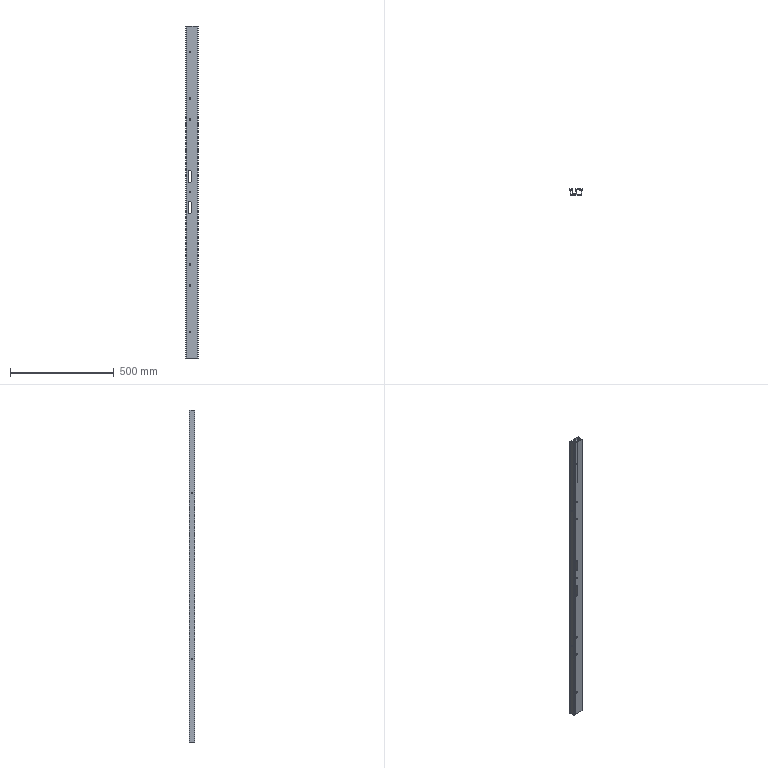Part | 2 solids | 121 faces | box 60 x 27.5 x 1600 mm | volume 628588 mm3 | cylinder 66 | plane 55 | commonest cylinder face diameters 7 x28 11 x12 2 x11 1 x4 4 x4 5 x4